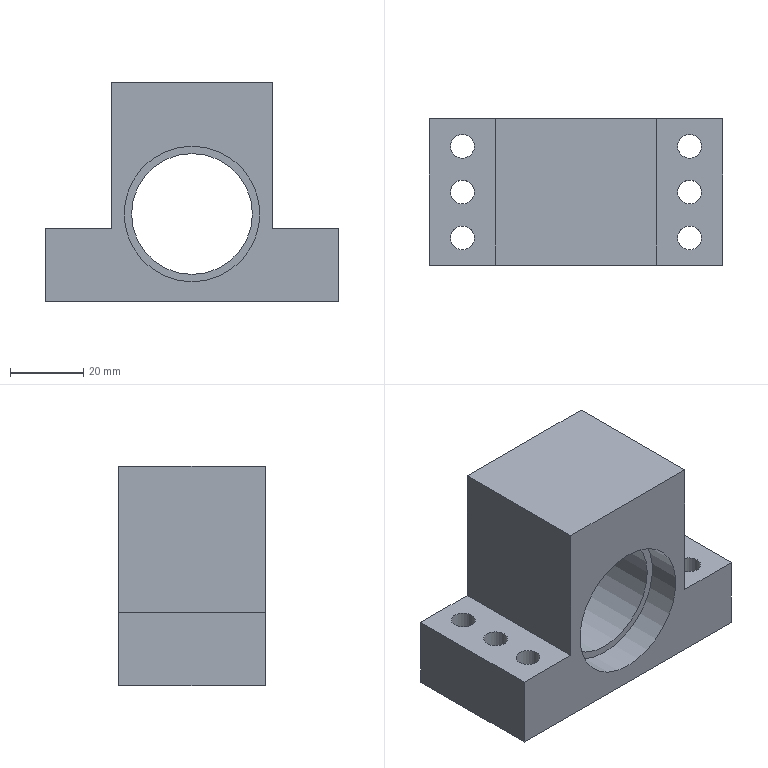Part | NX | features SIMPLE HOLE 6, DATUM_CSYS 5, SKETCH 4, EXTRUDE 2, HOLE PACKAGE 2, CBORE_HOLE 1 | 1 solid | 19 faces | box 80 x 40 x 60 mm | volume 94227 mm3 | plane 11 | cylinder 8 | commonest cylinder face diameters 6.5 x6 33 x1 37 x1
STEP:
#1=CARTESIAN_POINT('',(22.,20.,30.));
#2=VERTEX_POINT('',#1);
#3=CARTESIAN_POINT('',(22.,-20.,30.));
#4=VERTEX_POINT('',#3);
#5=CARTESIAN_POINT('',(22.,24.,30.));
#6=DIRECTION('',(0.,-1.,0.));
#7=VECTOR('',#6,1000.);
#8=LINE('',#5,#7);
#9=EDGE_CURVE('',#2,#4,#8,.T.);
#10=ORIENTED_EDGE('',*,*,#9,.F.);
#11=CARTESIAN_POINT('',(-22.,20.,30.));
#12=VERTEX_POINT('',#11);
#13=CARTESIAN_POINT('',(40.,20.,30.));
#14=DIRECTION('',(-1.,0.,0.));
#15=VECTOR('',#14,1000.);
#16=LINE('',#13,#15);
#17=EDGE_CURVE('',#2,#12,#16,.T.);
#18=ORIENTED_EDGE('',*,*,#17,.T.);
#19=CARTESIAN_POINT('',(-22.,-20.,30.));
#20=VERTEX_POINT('',#19);
#21=CARTESIAN_POINT('',(-22.,24.,30.));
#22=DIRECTION('',(0.,-1.,0.));
#23=VECTOR('',#22,1000.);
#24=LINE('',#21,#23);
#25=EDGE_CURVE('',#12,#20,#24,.T.);
#26=ORIENTED_EDGE('',*,*,#25,.T.);
#27=CARTESIAN_POINT('',(40.,-20.,30.));
#28=DIRECTION('',(-1.,0.,0.));
#29=VECTOR('',#28,1000.);
#30=LINE('',#27,#29);
#31=EDGE_CURVE('',#4,#20,#30,.T.);
#32=ORIENTED_EDGE('',*,*,#31,.F.);
#33=EDGE_LOOP('',(#10,#18,#26,#32));
#34=FACE_BOUND('',#33,.T.);
#35=CARTESIAN_POINT('',(40.,-20.,30.));
#36=DIRECTION('',(0.,0.,-1.));
#37=DIRECTION('',(-1.,0.,0.));
#38=AXIS2_PLACEMENT_3D('',#35,#36,#37);
#39=PLANE('',#38);
#40=ADVANCED_FACE('',(#34),#39,.F.);
#41=CARTESIAN_POINT('',(-40.,20.,-10.));
#42=VERTEX_POINT('',#41);
#43=CARTESIAN_POINT('',(-40.,-20.,-10.));
#44=VERTEX_POINT('',#43);
#45=CARTESIAN_POINT('',(-40.,24.,-10.));
#46=DIRECTION('',(0.,-1.,0.));
#47=VECTOR('',#46,1000.);
#48=LINE('',#45,#47);
#49=EDGE_CURVE('',#42,#44,#48,.T.);
#50=ORIENTED_EDGE('',*,*,#49,.F.);
#51=CARTESIAN_POINT('',(-40.,20.,-30.));
#52=VERTEX_POINT('',#51);
#53=CARTESIAN_POINT('',(-40.,20.,30.));
#54=DIRECTION('',(0.,0.,-1.));
#55=VECTOR('',#54,1000.);
#56=LINE('',#53,#55);
#57=EDGE_CURVE('',#42,#52,#56,.T.);
#58=ORIENTED_EDGE('',*,*,#57,.T.);
#59=CARTESIAN_POINT('',(-40.,-20.,-30.));
#60=VERTEX_POINT('',#59);
#61=CARTESIAN_POINT('',(-40.,-20.,-30.));
#62=DIRECTION('',(0.,1.,0.));
#63=VECTOR('',#62,1000.);
#64=LINE('',#61,#63);
#65=EDGE_CURVE('',#60,#52,#64,.T.);
#66=ORIENTED_EDGE('',*,*,#65,.F.);
#67=CARTESIAN_POINT('',(-40.,-20.,30.));
#68=DIRECTION('',(0.,0.,-1.));
#69=VECTOR('',#68,1000.);
#70=LINE('',#67,#69);
#71=EDGE_CURVE('',#44,#60,#70,.T.);
#72=ORIENTED_EDGE('',*,*,#71,.F.);
#73=EDGE_LOOP('',(#50,#58,#66,#72));
#74=FACE_BOUND('',#73,.T.);
#75=CARTESIAN_POINT('',(-40.,-20.,30.));
#76=DIRECTION('',(1.,0.,0.));
#77=DIRECTION('',(0.,0.,-1.));
#78=AXIS2_PLACEMENT_3D('',#75,#76,#77);
#79=PLANE('',#78);
#80=ADVANCED_FACE('',(#74),#79,.F.);
#81=CARTESIAN_POINT('',(34.25,-12.5,-30.));
#82=VERTEX_POINT('',#81);
#83=CARTESIAN_POINT('',(31.,-12.5,-30.));
#84=DIRECTION('',(0.,0.,1.));
#85=DIRECTION('',(1.,0.,0.));
#86=AXIS2_PLACEMENT_3D('',#83,#84,#85);
#87=CIRCLE('',#86,3.25);
#88=EDGE_CURVE('',#82,#82,#87,.T.);
#89=ORIENTED_EDGE('',*,*,#88,.T.);
#90=EDGE_LOOP('',(#89));
#91=FACE_BOUND('',#90,.T.);
#92=CARTESIAN_POINT('',(34.25,0.,-30.));
#93=VERTEX_POINT('',#92);
#94=CARTESIAN_POINT('',(31.,0.,-30.));
#95=DIRECTION('',(0.,0.,1.));
#96=DIRECTION('',(1.,0.,0.));
#97=AXIS2_PLACEMENT_3D('',#94,#95,#96);
#98=CIRCLE('',#97,3.25);
#99=EDGE_CURVE('',#93,#93,#98,.T.);
#100=ORIENTED_EDGE('',*,*,#99,.T.);
#101=EDGE_LOOP('',(#100));
#102=FACE_BOUND('',#101,.T.);
#103=CARTESIAN_POINT('',(34.25,12.5,-30.));
#104=VERTEX_POINT('',#103);
#105=CARTESIAN_POINT('',(31.,12.5,-30.));
#106=DIRECTION('',(0.,0.,1.));
#107=DIRECTION('',(1.,0.,0.));
#108=AXIS2_PLACEMENT_3D('',#105,#106,#107);
#109=CIRCLE('',#108,3.25);
#110=EDGE_CURVE('',#104,#104,#109,.T.);
#111=ORIENTED_EDGE('',*,*,#110,.T.);
#112=EDGE_LOOP('',(#111));
#113=FACE_BOUND('',#112,.T.);
#114=CARTESIAN_POINT('',(-27.75,12.5,-30.));
#115=VERTEX_POINT('',#114);
#116=CARTESIAN_POINT('',(-31.,12.5,-30.));
#117=DIRECTION('',(0.,0.,1.));
#118=DIRECTION('',(1.,0.,0.));
#119=AXIS2_PLACEMENT_3D('',#116,#117,#118);
#120=CIRCLE('',#119,3.25);
#121=EDGE_CURVE('',#115,#115,#120,.T.);
#122=ORIENTED_EDGE('',*,*,#121,.T.);
#123=EDGE_LOOP('',(#122));
#124=FACE_BOUND('',#123,.T.);
#125=CARTESIAN_POINT('',(-27.75,0.,-30.));
#126=VERTEX_POINT('',#125);
#127=CARTESIAN_POINT('',(-31.,0.,-30.));
#128=DIRECTION('',(0.,0.,1.));
#129=DIRECTION('',(1.,0.,0.));
#130=AXIS2_PLACEMENT_3D('',#127,#128,#129);
#131=CIRCLE('',#130,3.25);
#132=EDGE_CURVE('',#126,#126,#131,.T.);
#133=ORIENTED_EDGE('',*,*,#132,.T.);
#134=EDGE_LOOP('',(#133));
#135=FACE_BOUND('',#134,.T.);
#136=CARTESIAN_POINT('',(-27.75,-12.5,-30.));
#137=VERTEX_POINT('',#136);
#138=CARTESIAN_POINT('',(-31.,-12.5,-30.));
#139=DIRECTION('',(0.,0.,1.));
#140=DIRECTION('',(1.,0.,0.));
#141=AXIS2_PLACEMENT_3D('',#138,#139,#140);
#142=CIRCLE('',#141,3.25);
#143=EDGE_CURVE('',#137,#137,#142,.T.);
#144=ORIENTED_EDGE('',*,*,#143,.T.);
#145=EDGE_LOOP('',(#144));
#146=FACE_BOUND('',#145,.T.);
#147=CARTESIAN_POINT('',(40.,20.,-30.));
#148=VERTEX_POINT('',#147);
#149=CARTESIAN_POINT('',(-40.,20.,-30.));
#150=DIRECTION('',(1.,0.,0.));
#151=VECTOR('',#150,1000.);
#152=LINE('',#149,#151);
#153=EDGE_CURVE('',#52,#148,#152,.T.);
#154=ORIENTED_EDGE('',*,*,#153,.T.);
#155=CARTESIAN_POINT('',(40.,-20.,-30.));
#156=VERTEX_POINT('',#155);
#157=CARTESIAN_POINT('',(40.,-20.,-30.));
#158=DIRECTION('',(0.,1.,0.));
#159=VECTOR('',#158,1000.);
#160=LINE('',#157,#159);
#161=EDGE_CURVE('',#156,#148,#160,.T.);
#162=ORIENTED_EDGE('',*,*,#161,.F.);
#163=CARTESIAN_POINT('',(-40.,-20.,-30.));
#164=DIRECTION('',(1.,0.,0.));
#165=VECTOR('',#164,1000.);
#166=LINE('',#163,#165);
#167=EDGE_CURVE('',#60,#156,#166,.T.);
#168=ORIENTED_EDGE('',*,*,#167,.F.);
#169=ORIENTED_EDGE('',*,*,#65,.T.);
#170=EDGE_LOOP('',(#154,#162,#168,#169));
#171=FACE_BOUND('',#170,.T.);
#172=CARTESIAN_POINT('',(-40.,-20.,-30.));
#173=DIRECTION('',(0.,0.,1.));
#174=DIRECTION('',(1.,0.,0.));
#175=AXIS2_PLACEMENT_3D('',#172,#173,#174);
#176=PLANE('',#175);
#177=ADVANCED_FACE('',(#91,#102,#113,#124,#135,#146,#171),#176,.F.);
#178=CARTESIAN_POINT('',(40.,20.,-10.));
#179=VERTEX_POINT('',#178);
#180=CARTESIAN_POINT('',(40.,20.,-30.));
#181=DIRECTION('',(0.,0.,1.));
#182=VECTOR('',#181,1000.);
#183=LINE('',#180,#182);
#184=EDGE_CURVE('',#148,#179,#183,.T.);
#185=ORIENTED_EDGE('',*,*,#184,.T.);
#186=CARTESIAN_POINT('',(40.,-20.,-10.));
#187=VERTEX_POINT('',#186);
#188=CARTESIAN_POINT('',(40.,24.,-10.));
#189=DIRECTION('',(0.,-1.,0.));
#190=VECTOR('',#189,1000.);
#191=LINE('',#188,#190);
#192=EDGE_CURVE('',#179,#187,#191,.T.);
#193=ORIENTED_EDGE('',*,*,#192,.T.);
#194=CARTESIAN_POINT('',(40.,-20.,-30.));
#195=DIRECTION('',(0.,0.,1.));
#196=VECTOR('',#195,1000.);
#197=LINE('',#194,#196);
#198=EDGE_CURVE('',#156,#187,#197,.T.);
#199=ORIENTED_EDGE('',*,*,#198,.F.);
#200=ORIENTED_EDGE('',*,*,#161,.T.);
#201=EDGE_LOOP('',(#185,#193,#199,#200));
#202=FACE_BOUND('',#201,.T.);
#203=CARTESIAN_POINT('',(40.,-20.,-30.));
#204=DIRECTION('',(-1.,0.,0.));
#205=DIRECTION('',(0.,0.,1.));
#206=AXIS2_PLACEMENT_3D('',#203,#204,#205);
#207=PLANE('',#206);
#208=ADVANCED_FACE('',(#202),#207,.F.);
#209=CARTESIAN_POINT('',(22.,-20.,-10.));
#210=VERTEX_POINT('',#209);
#211=CARTESIAN_POINT('',(22.,-20.,30.));
#212=DIRECTION('',(0.,0.,-1.));
#213=VECTOR('',#212,1000.);
#214=LINE('',#211,#213);
#215=EDGE_CURVE('',#4,#210,#214,.T.);
#216=ORIENTED_EDGE('',*,*,#215,.F.);
#217=ORIENTED_EDGE('',*,*,#31,.T.);
#218=CARTESIAN_POINT('',(-22.,-20.,-10.));
#219=VERTEX_POINT('',#218);
#220=CARTESIAN_POINT('',(-22.,-20.,-10.));
#221=DIRECTION('',(0.,0.,1.));
#222=VECTOR('',#221,1000.);
#223=LINE('',#220,#222);
#224=EDGE_CURVE('',#219,#20,#223,.T.);
#225=ORIENTED_EDGE('',*,*,#224,.F.);
#226=CARTESIAN_POINT('',(-40.,-20.,-10.));
#227=DIRECTION('',(1.,0.,0.));
#228=VECTOR('',#227,1000.);
#229=LINE('',#226,#228);
#230=EDGE_CURVE('',#44,#219,#229,.T.);
#231=ORIENTED_EDGE('',*,*,#230,.F.);
#232=ORIENTED_EDGE('',*,*,#71,.T.);
#233=ORIENTED_EDGE('',*,*,#167,.T.);
#234=ORIENTED_EDGE('',*,*,#198,.T.);
#235=CARTESIAN_POINT('',(22.,-20.,-10.));
#236=DIRECTION('',(1.,0.,0.));
#237=VECTOR('',#236,1000.);
#238=LINE('',#235,#237);
#239=EDGE_CURVE('',#210,#187,#238,.T.);
#240=ORIENTED_EDGE('',*,*,#239,.F.);
#241=EDGE_LOOP('',(#216,#217,#225,#231,#232,#233,#234,#240));
#242=FACE_BOUND('',#241,.T.);
#243=CARTESIAN_POINT('',(0.,-20.,12.5));
#244=VERTEX_POINT('',#243);
#245=CARTESIAN_POINT('',(0.,-20.,-6.));
#246=DIRECTION('',(0.,1.,0.));
#247=DIRECTION('',(0.,0.,1.));
#248=AXIS2_PLACEMENT_3D('',#245,#246,#247);
#249=CIRCLE('',#248,18.5);
#250=EDGE_CURVE('',#244,#244,#249,.T.);
#251=ORIENTED_EDGE('',*,*,#250,.T.);
#252=EDGE_LOOP('',(#251));
#253=FACE_BOUND('',#252,.T.);
#254=CARTESIAN_POINT('',(0.,-20.,0.));
#255=DIRECTION('',(0.,-1.,0.));
#256=DIRECTION('',(0.,0.,-1.));
#257=AXIS2_PLACEMENT_3D('',#254,#255,#256);
#258=PLANE('',#257);
#259=ADVANCED_FACE('',(#242,#253),#258,.T.);
#260=CARTESIAN_POINT('',(0.,20.,-22.5));
#261=VERTEX_POINT('',#260);
#262=CARTESIAN_POINT('',(0.,20.,-6.));
#263=DIRECTION('',(0.,-1.,0.));
#264=DIRECTION('',(0.,0.,-1.));
#265=AXIS2_PLACEMENT_3D('',#262,#263,#264);
#266=CIRCLE('',#265,16.5);
#267=EDGE_CURVE('',#261,#261,#266,.T.);
#268=ORIENTED_EDGE('',*,*,#267,.T.);
#269=EDGE_LOOP('',(#268));
#270=FACE_BOUND('',#269,.T.);
#271=ORIENTED_EDGE('',*,*,#17,.F.);
#272=CARTESIAN_POINT('',(22.,20.,-10.));
#273=VERTEX_POINT('',#272);
#274=CARTESIAN_POINT('',(22.,20.,0.));
#275=DIRECTION('',(0.,0.,-1.));
#276=VECTOR('',#275,1000.);
#277=LINE('',#274,#276);
#278=EDGE_CURVE('',#2,#273,#277,.T.);
#279=ORIENTED_EDGE('',*,*,#278,.T.);
#280=CARTESIAN_POINT('',(0.,20.,-10.));
#281=DIRECTION('',(1.,0.,0.));
#282=VECTOR('',#281,1000.);
#283=LINE('',#280,#282);
#284=EDGE_CURVE('',#273,#179,#283,.T.);
#285=ORIENTED_EDGE('',*,*,#284,.T.);
#286=ORIENTED_EDGE('',*,*,#184,.F.);
#287=ORIENTED_EDGE('',*,*,#153,.F.);
#288=ORIENTED_EDGE('',*,*,#57,.F.);
#289=CARTESIAN_POINT('',(-22.,20.,-10.));
#290=VERTEX_POINT('',#289);
#291=CARTESIAN_POINT('',(0.,20.,-10.));
#292=DIRECTION('',(1.,0.,0.));
#293=VECTOR('',#292,1000.);
#294=LINE('',#291,#293);
#295=EDGE_CURVE('',#42,#290,#294,.T.);
#296=ORIENTED_EDGE('',*,*,#295,.T.);
#297=CARTESIAN_POINT('',(-22.,20.,0.));
#298=DIRECTION('',(0.,0.,1.));
#299=VECTOR('',#298,1000.);
#300=LINE('',#297,#299);
#301=EDGE_CURVE('',#290,#12,#300,.T.);
#302=ORIENTED_EDGE('',*,*,#301,.T.);
#303=EDGE_LOOP('',(#271,#279,#285,#286,#287,#288,#296,#302));
#304=FACE_BOUND('',#303,.T.);
#305=CARTESIAN_POINT('',(0.,20.,0.));
#306=DIRECTION('',(0.,-1.,0.));
#307=DIRECTION('',(0.,0.,-1.));
#308=AXIS2_PLACEMENT_3D('',#305,#306,#307);
#309=PLANE('',#308);
#310=ADVANCED_FACE('',(#270,#304),#309,.F.);
#311=CARTESIAN_POINT('',(0.,-11.,10.5));
#312=VERTEX_POINT('',#311);
#313=CARTESIAN_POINT('',(0.,-11.,-6.));
#314=DIRECTION('',(0.,1.,0.));
#315=DIRECTION('',(0.,0.,1.));
#316=AXIS2_PLACEMENT_3D('',#313,#314,#315);
#317=CIRCLE('',#316,16.5);
#318=EDGE_CURVE('',#312,#312,#317,.F.);
#319=ORIENTED_EDGE('',*,*,#318,.T.);
#320=EDGE_LOOP('',(#319));
#321=FACE_BOUND('',#320,.T.);
#322=ORIENTED_EDGE('',*,*,#267,.F.);
#323=EDGE_LOOP('',(#322));
#324=FACE_BOUND('',#323,.T.);
#325=CARTESIAN_POINT('',(0.,58.932,-6.));
#326=DIRECTION('',(0.,1.,0.));
#327=DIRECTION('',(0.,0.,1.));
#328=AXIS2_PLACEMENT_3D('',#325,#326,#327);
#329=CYLINDRICAL_SURFACE('',#328,16.5);
#330=ADVANCED_FACE('',(#321,#324),#329,.F.);
#331=ORIENTED_EDGE('',*,*,#318,.F.);
#332=EDGE_LOOP('',(#331));
#333=FACE_BOUND('',#332,.T.);
#334=CARTESIAN_POINT('',(0.,-11.,12.5));
#335=VERTEX_POINT('',#334);
#336=CARTESIAN_POINT('',(0.,-11.,-6.));
#337=DIRECTION('',(0.,1.,0.));
#338=DIRECTION('',(0.,0.,1.));
#339=AXIS2_PLACEMENT_3D('',#336,#337,#338);
#340=CIRCLE('',#339,18.5);
#341=EDGE_CURVE('',#335,#335,#340,.F.);
#342=ORIENTED_EDGE('',*,*,#341,.T.);
#343=EDGE_LOOP('',(#342));
#344=FACE_BOUND('',#343,.T.);
#345=CARTESIAN_POINT('',(0.,-11.,-6.));
#346=DIRECTION('',(0.,1.,0.));
#347=DIRECTION('',(0.,0.,1.));
#348=AXIS2_PLACEMENT_3D('',#345,#346,#347);
#349=PLANE('',#348);
#350=ADVANCED_FACE('',(#333,#344),#349,.F.);
#351=ORIENTED_EDGE('',*,*,#341,.F.);
#352=EDGE_LOOP('',(#351));
#353=FACE_BOUND('',#352,.T.);
#354=ORIENTED_EDGE('',*,*,#250,.F.);
#355=EDGE_LOOP('',(#354));
#356=FACE_BOUND('',#355,.T.);
#357=CARTESIAN_POINT('',(0.,-20.,-6.));
#358=DIRECTION('',(0.,1.,0.));
#359=DIRECTION('',(0.,0.,1.));
#360=AXIS2_PLACEMENT_3D('',#357,#358,#359);
#361=CYLINDRICAL_SURFACE('',#360,18.5);
#362=ADVANCED_FACE('',(#353,#356),#361,.F.);
#363=CARTESIAN_POINT('',(-34.25,12.5,-10.));
#364=VERTEX_POINT('',#363);
#365=CARTESIAN_POINT('',(-31.,12.5,-10.));
#366=DIRECTION('',(0.,0.,-1.));
#367=DIRECTION('',(-1.,0.,0.));
#368=AXIS2_PLACEMENT_3D('',#365,#366,#367);
#369=CIRCLE('',#368,3.25);
#370=EDGE_CURVE('',#364,#364,#369,.T.);
#371=ORIENTED_EDGE('',*,*,#370,.T.);
#372=EDGE_LOOP('',(#371));
#373=FACE_BOUND('',#372,.T.);
#374=CARTESIAN_POINT('',(-34.25,0.,-10.));
#375=VERTEX_POINT('',#374);
#376=CARTESIAN_POINT('',(-31.,0.,-10.));
#377=DIRECTION('',(0.,0.,-1.));
#378=DIRECTION('',(-1.,0.,0.));
#379=AXIS2_PLACEMENT_3D('',#376,#377,#378);
#380=CIRCLE('',#379,3.25);
#381=EDGE_CURVE('',#375,#375,#380,.T.);
#382=ORIENTED_EDGE('',*,*,#381,.T.);
#383=EDGE_LOOP('',(#382));
#384=FACE_BOUND('',#383,.T.);
#385=CARTESIAN_POINT('',(-34.25,-12.5,-10.));
#386=VERTEX_POINT('',#385);
#387=CARTESIAN_POINT('',(-31.,-12.5,-10.));
#388=DIRECTION('',(0.,0.,-1.));
#389=DIRECTION('',(-1.,0.,0.));
#390=AXIS2_PLACEMENT_3D('',#387,#388,#389);
#391=CIRCLE('',#390,3.25);
#392=EDGE_CURVE('',#386,#386,#391,.T.);
#393=ORIENTED_EDGE('',*,*,#392,.T.);
#394=EDGE_LOOP('',(#393));
#395=FACE_BOUND('',#394,.T.);
#396=ORIENTED_EDGE('',*,*,#49,.T.);
#397=ORIENTED_EDGE('',*,*,#230,.T.);
#398=CARTESIAN_POINT('',(-22.,24.,-10.));
#399=DIRECTION('',(0.,-1.,0.));
#400=VECTOR('',#399,1000.);
#401=LINE('',#398,#400);
#402=EDGE_CURVE('',#219,#290,#401,.F.);
#403=ORIENTED_EDGE('',*,*,#402,.T.);
#404=ORIENTED_EDGE('',*,*,#295,.F.);
#405=EDGE_LOOP('',(#396,#397,#403,#404));
#406=FACE_BOUND('',#405,.T.);
#407=CARTESIAN_POINT('',(-40.,24.,-10.));
#408=DIRECTION('',(0.,0.,-1.));
#409=DIRECTION('',(-1.,0.,0.));
#410=AXIS2_PLACEMENT_3D('',#407,#408,#409);
#411=PLANE('',#410);
#412=ADVANCED_FACE('',(#373,#384,#395,#406),#411,.F.);
#413=ORIENTED_EDGE('',*,*,#402,.F.);
#414=ORIENTED_EDGE('',*,*,#224,.T.);
#415=ORIENTED_EDGE('',*,*,#25,.F.);
#416=ORIENTED_EDGE('',*,*,#301,.F.);
#417=EDGE_LOOP('',(#413,#414,#415,#416));
#418=FACE_BOUND('',#417,.T.);
#419=CARTESIAN_POINT('',(-22.,24.,-10.));
#420=DIRECTION('',(1.,0.,0.));
#421=DIRECTION('',(0.,0.,-1.));
#422=AXIS2_PLACEMENT_3D('',#419,#420,#421);
#423=PLANE('',#422);
#424=ADVANCED_FACE('',(#418),#423,.F.);
#425=ORIENTED_EDGE('',*,*,#9,.T.);
#426=ORIENTED_EDGE('',*,*,#215,.T.);
#427=CARTESIAN_POINT('',(22.,24.,-10.));
#428=DIRECTION('',(0.,-1.,0.));
#429=VECTOR('',#428,1000.);
#430=LINE('',#427,#429);
#431=EDGE_CURVE('',#210,#273,#430,.F.);
#432=ORIENTED_EDGE('',*,*,#431,.T.);
#433=ORIENTED_EDGE('',*,*,#278,.F.);
#434=EDGE_LOOP('',(#425,#426,#432,#433));
#435=FACE_BOUND('',#434,.T.);
#436=CARTESIAN_POINT('',(22.,24.,30.));
#437=DIRECTION('',(-1.,0.,0.));
#438=DIRECTION('',(0.,0.,1.));
#439=AXIS2_PLACEMENT_3D('',#436,#437,#438);
#440=PLANE('',#439);
#441=ADVANCED_FACE('',(#435),#440,.F.);
#442=CARTESIAN_POINT('',(27.75,-12.5,-10.));
#443=VERTEX_POINT('',#442);
#444=CARTESIAN_POINT('',(31.,-12.5,-10.));
#445=DIRECTION('',(0.,0.,-1.));
#446=DIRECTION('',(-1.,0.,0.));
#447=AXIS2_PLACEMENT_3D('',#444,#445,#446);
#448=CIRCLE('',#447,3.25);
#449=EDGE_CURVE('',#443,#443,#448,.T.);
#450=ORIENTED_EDGE('',*,*,#449,.T.);
#451=EDGE_LOOP('',(#450));
#452=FACE_BOUND('',#451,.T.);
#453=CARTESIAN_POINT('',(27.75,0.,-10.));
#454=VERTEX_POINT('',#453);
#455=CARTESIAN_POINT('',(31.,0.,-10.));
#456=DIRECTION('',(0.,0.,-1.));
#457=DIRECTION('',(-1.,0.,0.));
#458=AXIS2_PLACEMENT_3D('',#455,#456,#457);
#459=CIRCLE('',#458,3.25);
#460=EDGE_CURVE('',#454,#454,#459,.T.);
#461=ORIENTED_EDGE('',*,*,#460,.T.);
#462=EDGE_LOOP('',(#461));
#463=FACE_BOUND('',#462,.T.);
#464=CARTESIAN_POINT('',(27.75,12.5,-10.));
#465=VERTEX_POINT('',#464);
#466=CARTESIAN_POINT('',(31.,12.5,-10.));
#467=DIRECTION('',(0.,0.,-1.));
#468=DIRECTION('',(-1.,0.,0.));
#469=AXIS2_PLACEMENT_3D('',#466,#467,#468);
#470=CIRCLE('',#469,3.25);
#471=EDGE_CURVE('',#465,#465,#470,.T.);
#472=ORIENTED_EDGE('',*,*,#471,.T.);
#473=EDGE_LOOP('',(#472));
#474=FACE_BOUND('',#473,.T.);
#475=ORIENTED_EDGE('',*,*,#431,.F.);
#476=ORIENTED_EDGE('',*,*,#239,.T.);
#477=ORIENTED_EDGE('',*,*,#192,.F.);
#478=ORIENTED_EDGE('',*,*,#284,.F.);
#479=EDGE_LOOP('',(#475,#476,#477,#478));
#480=FACE_BOUND('',#479,.T.);
#481=CARTESIAN_POINT('',(22.,24.,-10.));
#482=DIRECTION('',(0.,0.,-1.));
#483=DIRECTION('',(-1.,0.,0.));
#484=AXIS2_PLACEMENT_3D('',#481,#482,#483);
#485=PLANE('',#484);
#486=ADVANCED_FACE('',(#452,#463,#474,#480),#485,.F.);
#487=ORIENTED_EDGE('',*,*,#392,.F.);
#488=EDGE_LOOP('',(#487));
#489=FACE_BOUND('',#488,.T.);
#490=ORIENTED_EDGE('',*,*,#143,.F.);
#491=EDGE_LOOP('',(#490));
#492=FACE_BOUND('',#491,.T.);
#493=CARTESIAN_POINT('',(-31.,-12.5,-10.));
#494=DIRECTION('',(0.,0.,-1.));
#495=DIRECTION('',(-1.,0.,0.));
#496=AXIS2_PLACEMENT_3D('',#493,#494,#495);
#497=CYLINDRICAL_SURFACE('',#496,3.25);
#498=ADVANCED_FACE('',(#489,#492),#497,.F.);
#499=ORIENTED_EDGE('',*,*,#381,.F.);
#500=EDGE_LOOP('',(#499));
#501=FACE_BOUND('',#500,.T.);
#502=ORIENTED_EDGE('',*,*,#132,.F.);
#503=EDGE_LOOP('',(#502));
#504=FACE_BOUND('',#503,.T.);
#505=CARTESIAN_POINT('',(-31.,0.,-10.));
#506=DIRECTION('',(0.,0.,-1.));
#507=DIRECTION('',(-1.,0.,0.));
#508=AXIS2_PLACEMENT_3D('',#505,#506,#507);
#509=CYLINDRICAL_SURFACE('',#508,3.25);
#510=ADVANCED_FACE('',(#501,#504),#509,.F.);
#511=ORIENTED_EDGE('',*,*,#370,.F.);
#512=EDGE_LOOP('',(#511));
#513=FACE_BOUND('',#512,.T.);
#514=ORIENTED_EDGE('',*,*,#121,.F.);
#515=EDGE_LOOP('',(#514));
#516=FACE_BOUND('',#515,.T.);
#517=CARTESIAN_POINT('',(-31.,12.5,-10.));
#518=DIRECTION('',(0.,0.,-1.));
#519=DIRECTION('',(-1.,0.,0.));
#520=AXIS2_PLACEMENT_3D('',#517,#518,#519);
#521=CYLINDRICAL_SURFACE('',#520,3.25);
#522=ADVANCED_FACE('',(#513,#516),#521,.F.);
#523=ORIENTED_EDGE('',*,*,#471,.F.);
#524=EDGE_LOOP('',(#523));
#525=FACE_BOUND('',#524,.T.);
#526=ORIENTED_EDGE('',*,*,#110,.F.);
#527=EDGE_LOOP('',(#526));
#528=FACE_BOUND('',#527,.T.);
#529=CARTESIAN_POINT('',(31.,12.5,-10.));
#530=DIRECTION('',(0.,0.,-1.));
#531=DIRECTION('',(-1.,0.,0.));
#532=AXIS2_PLACEMENT_3D('',#529,#530,#531);
#533=CYLINDRICAL_SURFACE('',#532,3.25);
#534=ADVANCED_FACE('',(#525,#528),#533,.F.);
#535=ORIENTED_EDGE('',*,*,#460,.F.);
#536=EDGE_LOOP('',(#535));
#537=FACE_BOUND('',#536,.T.);
#538=ORIENTED_EDGE('',*,*,#99,.F.);
#539=EDGE_LOOP('',(#538));
#540=FACE_BOUND('',#539,.T.);
#541=CARTESIAN_POINT('',(31.,0.,-10.));
#542=DIRECTION('',(0.,0.,-1.));
#543=DIRECTION('',(-1.,0.,0.));
#544=AXIS2_PLACEMENT_3D('',#541,#542,#543);
#545=CYLINDRICAL_SURFACE('',#544,3.25);
#546=ADVANCED_FACE('',(#537,#540),#545,.F.);
#547=ORIENTED_EDGE('',*,*,#449,.F.);
#548=EDGE_LOOP('',(#547));
#549=FACE_BOUND('',#548,.T.);
#550=ORIENTED_EDGE('',*,*,#88,.F.);
#551=EDGE_LOOP('',(#550));
#552=FACE_BOUND('',#551,.T.);
#553=CARTESIAN_POINT('',(31.,-12.5,-10.));
#554=DIRECTION('',(0.,0.,-1.));
#555=DIRECTION('',(-1.,0.,0.));
#556=AXIS2_PLACEMENT_3D('',#553,#554,#555);
#557=CYLINDRICAL_SURFACE('',#556,3.25);
#558=ADVANCED_FACE('',(#549,#552),#557,.F.);
#559=CLOSED_SHELL('',(#40,#80,#177,#208,#259,#310,#330,#350,#362,#412,#424,#441,#486,#498,#510,#522,#534,#546,#558));
#560=MANIFOLD_SOLID_BREP('',#559);
#561=(LENGTH_UNIT()NAMED_UNIT(*)SI_UNIT(.MILLI.,.METRE.));
#562=UNCERTAINTY_MEASURE_WITH_UNIT(LENGTH_MEASURE(0.00001),#561,'','');
#563=(NAMED_UNIT(*)PLANE_ANGLE_UNIT()SI_UNIT($,.RADIAN.));
#564=(NAMED_UNIT(*)SI_UNIT($,.STERADIAN.)SOLID_ANGLE_UNIT());
#565=(GEOMETRIC_REPRESENTATION_CONTEXT(3)GLOBAL_UNCERTAINTY_ASSIGNED_CONTEXT((#562))GLOBAL_UNIT_ASSIGNED_CONTEXT((#561,#563,#564))REPRESENTATION_CONTEXT('',''));
#566=ADVANCED_BREP_SHAPE_REPRESENTATION('',(#560),#565);